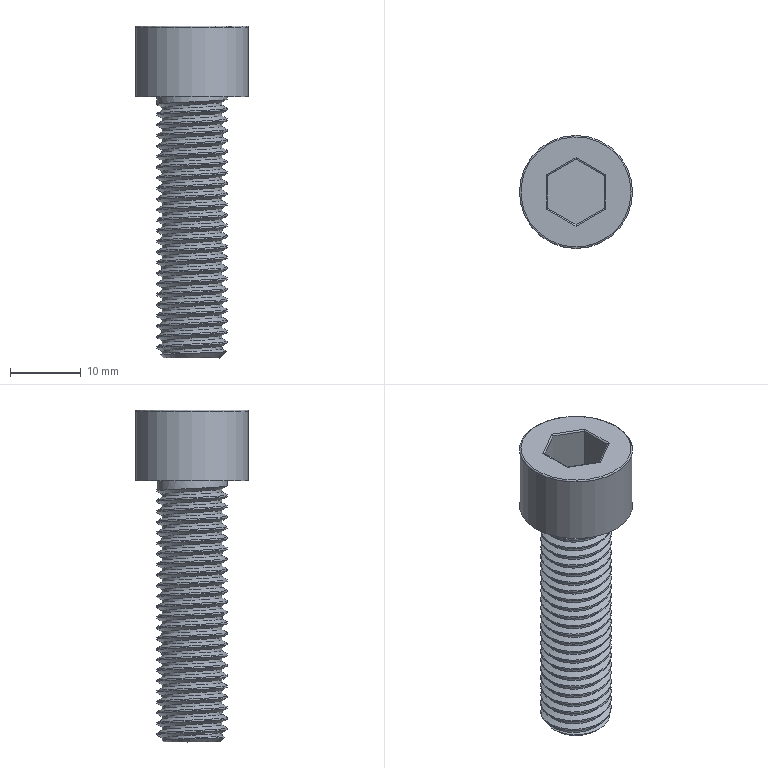Part | STEP file | Tube feed_id1550_x_t | 1 solid | 26 faces | box 16 x 16 x 47 mm | volume 4055 mm3 | plane 11 | cylinder 9 | spline 3 | cone 2 | torus 1 | commonest cylinder face diameters 0.4 x6 8.5 x1 10 x1 16 x1